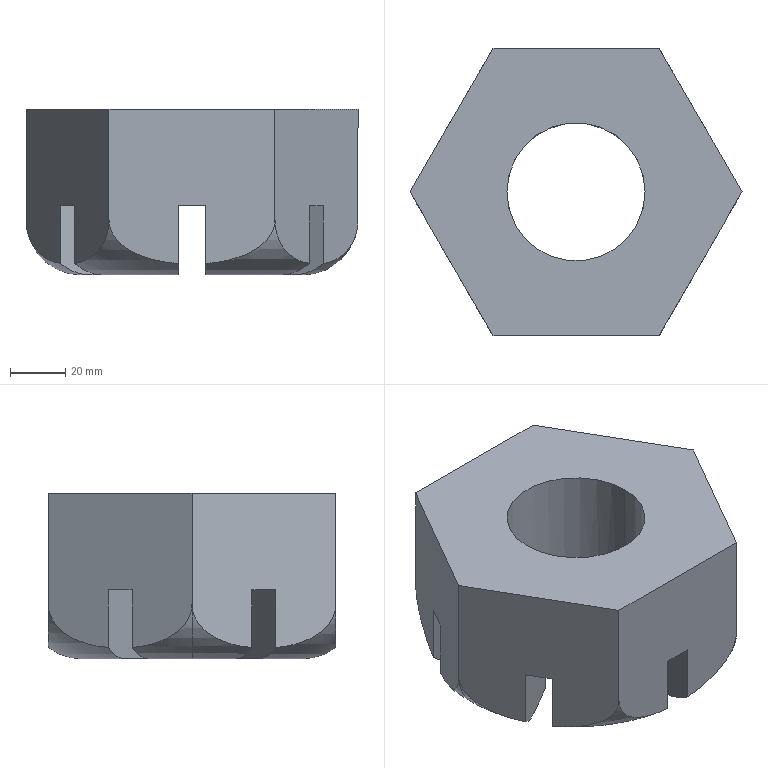Part | SolidWorks | features ICE 2, CirPattern 1, Extrusion 1, RevCut 1 | 1 solid | 40 faces | box 120.089 x 104 x 60 mm | volume 394121 mm3 | plane 31 | torus 7 | cylinder 2 | commonest cylinder face diameters 50 x2